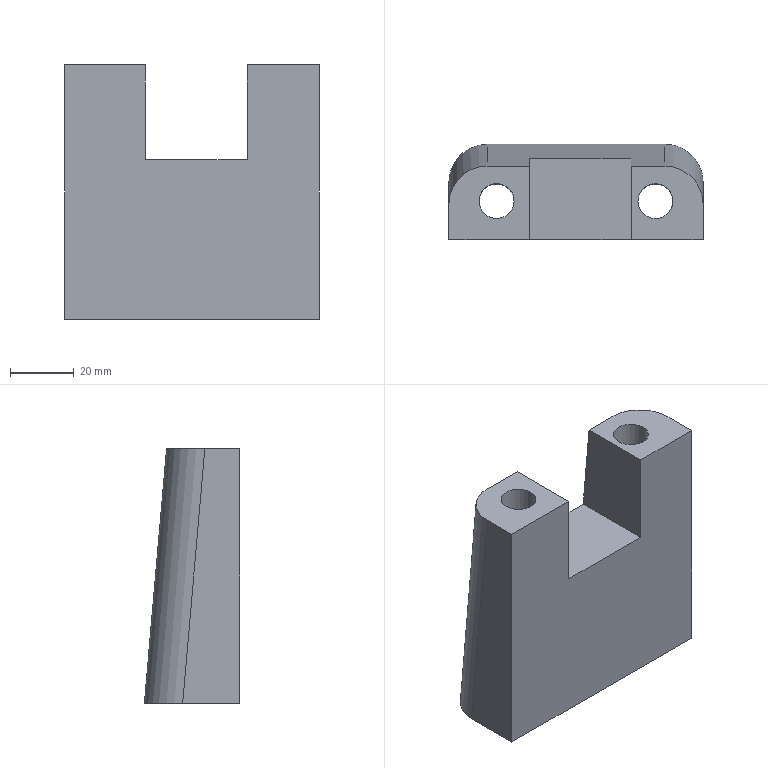Part | STEP file | solid 123 | 1 solid | 22 faces | box 80 x 30 x 80 mm | volume 120680 mm3 | plane 12 | cylinder 8 | cone 2 | commonest cylinder face diameters 11 x2 18 x2 24 x2 9 x1 10 x1